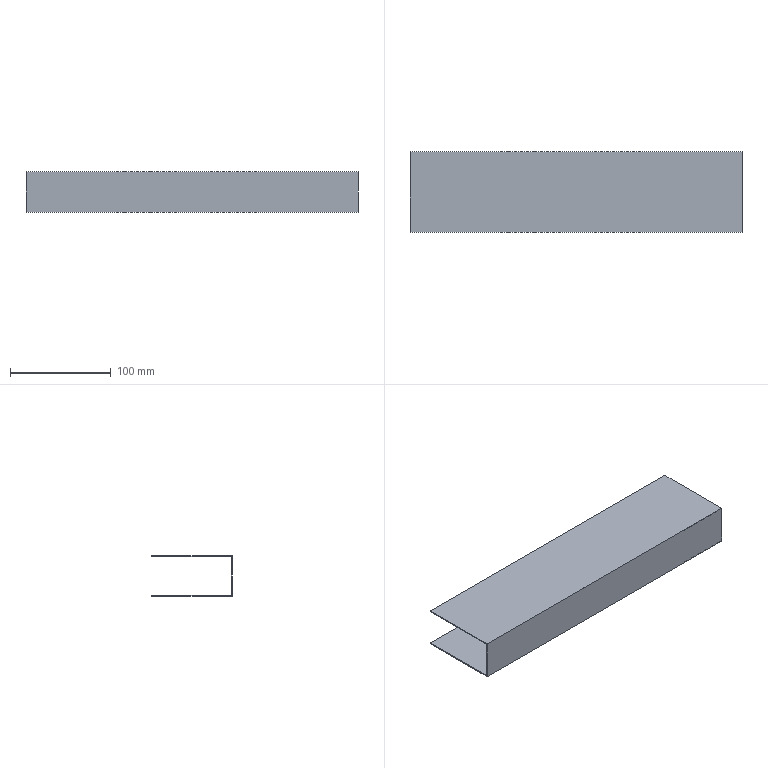Part | SolidWorks | features BaseBody 1 | 1 solid | 10 faces | box 330 x 80 x 40 mm | volume 65340 mm3 | plane 10
STEP:
#1=CARTESIAN_POINT('',(0.,1.,19.));
#2=VERTEX_POINT('',#1);
#3=CARTESIAN_POINT('',(0.,80.,19.));
#4=VERTEX_POINT('',#3);
#5=CARTESIAN_POINT('',(0.,0.,19.));
#6=DIRECTION('',(0.,1.,0.));
#7=VECTOR('',#6,1000.);
#8=LINE('',#5,#7);
#9=EDGE_CURVE('',#2,#4,#8,.T.);
#10=ORIENTED_EDGE('',*,*,#9,.F.);
#11=CARTESIAN_POINT('',(0.,1.,-19.));
#12=VERTEX_POINT('',#11);
#13=CARTESIAN_POINT('',(0.,1.,20.));
#14=DIRECTION('',(0.,0.,1.));
#15=VECTOR('',#14,1000.);
#16=LINE('',#13,#15);
#17=EDGE_CURVE('',#12,#2,#16,.T.);
#18=ORIENTED_EDGE('',*,*,#17,.F.);
#19=CARTESIAN_POINT('',(0.,80.,-19.));
#20=VERTEX_POINT('',#19);
#21=CARTESIAN_POINT('',(0.,0.,-19.));
#22=DIRECTION('',(0.,-1.,0.));
#23=VECTOR('',#22,1000.);
#24=LINE('',#21,#23);
#25=EDGE_CURVE('',#20,#12,#24,.T.);
#26=ORIENTED_EDGE('',*,*,#25,.F.);
#27=CARTESIAN_POINT('',(0.,80.,-20.));
#28=VERTEX_POINT('',#27);
#29=CARTESIAN_POINT('',(0.,80.,-19.));
#30=DIRECTION('',(0.,0.,-1.));
#31=VECTOR('',#30,1000.);
#32=LINE('',#29,#31);
#33=EDGE_CURVE('',#20,#28,#32,.T.);
#34=ORIENTED_EDGE('',*,*,#33,.T.);
#35=CARTESIAN_POINT('',(0.,0.,-20.));
#36=VERTEX_POINT('',#35);
#37=CARTESIAN_POINT('',(0.,0.,-20.));
#38=DIRECTION('',(0.,-1.,0.));
#39=VECTOR('',#38,1000.);
#40=LINE('',#37,#39);
#41=EDGE_CURVE('',#28,#36,#40,.T.);
#42=ORIENTED_EDGE('',*,*,#41,.T.);
#43=CARTESIAN_POINT('',(0.,0.,20.));
#44=VERTEX_POINT('',#43);
#45=CARTESIAN_POINT('',(0.,0.,20.));
#46=DIRECTION('',(0.,0.,1.));
#47=VECTOR('',#46,1000.);
#48=LINE('',#45,#47);
#49=EDGE_CURVE('',#36,#44,#48,.T.);
#50=ORIENTED_EDGE('',*,*,#49,.T.);
#51=CARTESIAN_POINT('',(0.,80.,20.));
#52=VERTEX_POINT('',#51);
#53=CARTESIAN_POINT('',(0.,0.,20.));
#54=DIRECTION('',(0.,1.,0.));
#55=VECTOR('',#54,1000.);
#56=LINE('',#53,#55);
#57=EDGE_CURVE('',#44,#52,#56,.T.);
#58=ORIENTED_EDGE('',*,*,#57,.T.);
#59=CARTESIAN_POINT('',(0.,80.,20.));
#60=DIRECTION('',(0.,0.,-1.));
#61=VECTOR('',#60,1000.);
#62=LINE('',#59,#61);
#63=EDGE_CURVE('',#52,#4,#62,.T.);
#64=ORIENTED_EDGE('',*,*,#63,.T.);
#65=EDGE_LOOP('',(#10,#18,#26,#34,#42,#50,#58,#64));
#66=FACE_OUTER_BOUND('',#65,.T.);
#67=CARTESIAN_POINT('',(0.,0.,0.));
#68=DIRECTION('',(-1.,0.,0.));
#69=DIRECTION('',(0.,0.,1.));
#70=AXIS2_PLACEMENT_3D('',#67,#68,#69);
#71=PLANE('',#70);
#72=ADVANCED_FACE('',(#66),#71,.T.);
#73=CARTESIAN_POINT('',(330.,1.,19.));
#74=VERTEX_POINT('',#73);
#75=CARTESIAN_POINT('',(330.,80.,19.));
#76=VERTEX_POINT('',#75);
#77=CARTESIAN_POINT('',(330.,0.,19.));
#78=DIRECTION('',(0.,1.,0.));
#79=VECTOR('',#78,1000.);
#80=LINE('',#77,#79);
#81=EDGE_CURVE('',#74,#76,#80,.T.);
#82=ORIENTED_EDGE('',*,*,#81,.T.);
#83=CARTESIAN_POINT('',(330.,80.,20.));
#84=VERTEX_POINT('',#83);
#85=CARTESIAN_POINT('',(330.,80.,20.));
#86=DIRECTION('',(0.,0.,-1.));
#87=VECTOR('',#86,1000.);
#88=LINE('',#85,#87);
#89=EDGE_CURVE('',#84,#76,#88,.T.);
#90=ORIENTED_EDGE('',*,*,#89,.F.);
#91=CARTESIAN_POINT('',(330.,0.,20.));
#92=VERTEX_POINT('',#91);
#93=CARTESIAN_POINT('',(330.,0.,20.));
#94=DIRECTION('',(0.,1.,0.));
#95=VECTOR('',#94,1000.);
#96=LINE('',#93,#95);
#97=EDGE_CURVE('',#92,#84,#96,.T.);
#98=ORIENTED_EDGE('',*,*,#97,.F.);
#99=CARTESIAN_POINT('',(330.,0.,-20.));
#100=VERTEX_POINT('',#99);
#101=CARTESIAN_POINT('',(330.,0.,20.));
#102=DIRECTION('',(0.,0.,1.));
#103=VECTOR('',#102,1000.);
#104=LINE('',#101,#103);
#105=EDGE_CURVE('',#100,#92,#104,.T.);
#106=ORIENTED_EDGE('',*,*,#105,.F.);
#107=CARTESIAN_POINT('',(330.,80.,-20.));
#108=VERTEX_POINT('',#107);
#109=CARTESIAN_POINT('',(330.,0.,-20.));
#110=DIRECTION('',(0.,-1.,0.));
#111=VECTOR('',#110,1000.);
#112=LINE('',#109,#111);
#113=EDGE_CURVE('',#108,#100,#112,.T.);
#114=ORIENTED_EDGE('',*,*,#113,.F.);
#115=CARTESIAN_POINT('',(330.,80.,-19.));
#116=VERTEX_POINT('',#115);
#117=CARTESIAN_POINT('',(330.,80.,-19.));
#118=DIRECTION('',(0.,0.,-1.));
#119=VECTOR('',#118,1000.);
#120=LINE('',#117,#119);
#121=EDGE_CURVE('',#116,#108,#120,.T.);
#122=ORIENTED_EDGE('',*,*,#121,.F.);
#123=CARTESIAN_POINT('',(330.,1.,-19.));
#124=VERTEX_POINT('',#123);
#125=CARTESIAN_POINT('',(330.,0.,-19.));
#126=DIRECTION('',(0.,-1.,0.));
#127=VECTOR('',#126,1000.);
#128=LINE('',#125,#127);
#129=EDGE_CURVE('',#116,#124,#128,.T.);
#130=ORIENTED_EDGE('',*,*,#129,.T.);
#131=CARTESIAN_POINT('',(330.,1.,20.));
#132=DIRECTION('',(0.,0.,1.));
#133=VECTOR('',#132,1000.);
#134=LINE('',#131,#133);
#135=EDGE_CURVE('',#124,#74,#134,.T.);
#136=ORIENTED_EDGE('',*,*,#135,.T.);
#137=EDGE_LOOP('',(#82,#90,#98,#106,#114,#122,#130,#136));
#138=FACE_OUTER_BOUND('',#137,.T.);
#139=CARTESIAN_POINT('',(330.,0.,0.));
#140=DIRECTION('',(-1.,0.,0.));
#141=DIRECTION('',(0.,0.,1.));
#142=AXIS2_PLACEMENT_3D('',#139,#140,#141);
#143=PLANE('',#142);
#144=ADVANCED_FACE('',(#138),#143,.F.);
#145=ORIENTED_EDGE('',*,*,#17,.T.);
#146=CARTESIAN_POINT('',(330.,1.,19.));
#147=DIRECTION('',(-1.,0.,0.));
#148=VECTOR('',#147,1000.);
#149=LINE('',#146,#148);
#150=EDGE_CURVE('',#74,#2,#149,.T.);
#151=ORIENTED_EDGE('',*,*,#150,.F.);
#152=ORIENTED_EDGE('',*,*,#135,.F.);
#153=CARTESIAN_POINT('',(330.,1.,-19.));
#154=DIRECTION('',(-1.,0.,0.));
#155=VECTOR('',#154,1000.);
#156=LINE('',#153,#155);
#157=EDGE_CURVE('',#124,#12,#156,.T.);
#158=ORIENTED_EDGE('',*,*,#157,.T.);
#159=EDGE_LOOP('',(#145,#151,#152,#158));
#160=FACE_OUTER_BOUND('',#159,.T.);
#161=CARTESIAN_POINT('',(330.,1.,20.));
#162=DIRECTION('',(0.,-1.,0.));
#163=DIRECTION('',(0.,0.,-1.));
#164=AXIS2_PLACEMENT_3D('',#161,#162,#163);
#165=PLANE('',#164);
#166=ADVANCED_FACE('',(#160),#165,.F.);
#167=ORIENTED_EDGE('',*,*,#25,.T.);
#168=ORIENTED_EDGE('',*,*,#157,.F.);
#169=ORIENTED_EDGE('',*,*,#129,.F.);
#170=CARTESIAN_POINT('',(330.,80.,-19.));
#171=DIRECTION('',(-1.,0.,0.));
#172=VECTOR('',#171,1000.);
#173=LINE('',#170,#172);
#174=EDGE_CURVE('',#116,#20,#173,.T.);
#175=ORIENTED_EDGE('',*,*,#174,.T.);
#176=EDGE_LOOP('',(#167,#168,#169,#175));
#177=FACE_OUTER_BOUND('',#176,.T.);
#178=CARTESIAN_POINT('',(330.,0.,-19.));
#179=DIRECTION('',(0.,0.,-1.));
#180=DIRECTION('',(0.,-1.,0.));
#181=AXIS2_PLACEMENT_3D('',#178,#179,#180);
#182=PLANE('',#181);
#183=ADVANCED_FACE('',(#177),#182,.F.);
#184=ORIENTED_EDGE('',*,*,#33,.F.);
#185=ORIENTED_EDGE('',*,*,#174,.F.);
#186=ORIENTED_EDGE('',*,*,#121,.T.);
#187=CARTESIAN_POINT('',(330.,80.,-20.));
#188=DIRECTION('',(-1.,0.,0.));
#189=VECTOR('',#188,1000.);
#190=LINE('',#187,#189);
#191=EDGE_CURVE('',#108,#28,#190,.T.);
#192=ORIENTED_EDGE('',*,*,#191,.T.);
#193=EDGE_LOOP('',(#184,#185,#186,#192));
#194=FACE_OUTER_BOUND('',#193,.T.);
#195=CARTESIAN_POINT('',(330.,80.,-19.));
#196=DIRECTION('',(0.,1.,0.));
#197=DIRECTION('',(1.,0.,0.));
#198=AXIS2_PLACEMENT_3D('',#195,#196,#197);
#199=PLANE('',#198);
#200=ADVANCED_FACE('',(#194),#199,.T.);
#201=ORIENTED_EDGE('',*,*,#41,.F.);
#202=ORIENTED_EDGE('',*,*,#191,.F.);
#203=ORIENTED_EDGE('',*,*,#113,.T.);
#204=CARTESIAN_POINT('',(330.,0.,-20.));
#205=DIRECTION('',(-1.,0.,0.));
#206=VECTOR('',#205,1000.);
#207=LINE('',#204,#206);
#208=EDGE_CURVE('',#100,#36,#207,.T.);
#209=ORIENTED_EDGE('',*,*,#208,.T.);
#210=EDGE_LOOP('',(#201,#202,#203,#209));
#211=FACE_OUTER_BOUND('',#210,.T.);
#212=CARTESIAN_POINT('',(330.,0.,-20.));
#213=DIRECTION('',(0.,0.,-1.));
#214=DIRECTION('',(0.,-1.,0.));
#215=AXIS2_PLACEMENT_3D('',#212,#213,#214);
#216=PLANE('',#215);
#217=ADVANCED_FACE('',(#211),#216,.T.);
#218=ORIENTED_EDGE('',*,*,#49,.F.);
#219=ORIENTED_EDGE('',*,*,#208,.F.);
#220=ORIENTED_EDGE('',*,*,#105,.T.);
#221=CARTESIAN_POINT('',(330.,0.,20.));
#222=DIRECTION('',(-1.,0.,0.));
#223=VECTOR('',#222,1000.);
#224=LINE('',#221,#223);
#225=EDGE_CURVE('',#92,#44,#224,.T.);
#226=ORIENTED_EDGE('',*,*,#225,.T.);
#227=EDGE_LOOP('',(#218,#219,#220,#226));
#228=FACE_OUTER_BOUND('',#227,.T.);
#229=CARTESIAN_POINT('',(330.,0.,20.));
#230=DIRECTION('',(0.,-1.,0.));
#231=DIRECTION('',(0.,0.,-1.));
#232=AXIS2_PLACEMENT_3D('',#229,#230,#231);
#233=PLANE('',#232);
#234=ADVANCED_FACE('',(#228),#233,.T.);
#235=ORIENTED_EDGE('',*,*,#57,.F.);
#236=ORIENTED_EDGE('',*,*,#225,.F.);
#237=ORIENTED_EDGE('',*,*,#97,.T.);
#238=CARTESIAN_POINT('',(330.,80.,20.));
#239=DIRECTION('',(-1.,0.,0.));
#240=VECTOR('',#239,1000.);
#241=LINE('',#238,#240);
#242=EDGE_CURVE('',#84,#52,#241,.T.);
#243=ORIENTED_EDGE('',*,*,#242,.T.);
#244=EDGE_LOOP('',(#235,#236,#237,#243));
#245=FACE_OUTER_BOUND('',#244,.T.);
#246=CARTESIAN_POINT('',(330.,0.,20.));
#247=DIRECTION('',(0.,0.,1.));
#248=DIRECTION('',(0.,-1.,0.));
#249=AXIS2_PLACEMENT_3D('',#246,#247,#248);
#250=PLANE('',#249);
#251=ADVANCED_FACE('',(#245),#250,.T.);
#252=ORIENTED_EDGE('',*,*,#63,.F.);
#253=ORIENTED_EDGE('',*,*,#242,.F.);
#254=ORIENTED_EDGE('',*,*,#89,.T.);
#255=CARTESIAN_POINT('',(330.,80.,19.));
#256=DIRECTION('',(-1.,0.,0.));
#257=VECTOR('',#256,1000.);
#258=LINE('',#255,#257);
#259=EDGE_CURVE('',#76,#4,#258,.T.);
#260=ORIENTED_EDGE('',*,*,#259,.T.);
#261=EDGE_LOOP('',(#252,#253,#254,#260));
#262=FACE_OUTER_BOUND('',#261,.T.);
#263=CARTESIAN_POINT('',(330.,80.,20.));
#264=DIRECTION('',(0.,1.,0.));
#265=DIRECTION('',(1.,0.,0.));
#266=AXIS2_PLACEMENT_3D('',#263,#264,#265);
#267=PLANE('',#266);
#268=ADVANCED_FACE('',(#262),#267,.T.);
#269=ORIENTED_EDGE('',*,*,#9,.T.);
#270=ORIENTED_EDGE('',*,*,#259,.F.);
#271=ORIENTED_EDGE('',*,*,#81,.F.);
#272=ORIENTED_EDGE('',*,*,#150,.T.);
#273=EDGE_LOOP('',(#269,#270,#271,#272));
#274=FACE_OUTER_BOUND('',#273,.T.);
#275=CARTESIAN_POINT('',(330.,0.,19.));
#276=DIRECTION('',(0.,0.,1.));
#277=DIRECTION('',(0.,-1.,0.));
#278=AXIS2_PLACEMENT_3D('',#275,#276,#277);
#279=PLANE('',#278);
#280=ADVANCED_FACE('',(#274),#279,.F.);
#281=CLOSED_SHELL('',(#72,#144,#166,#183,#200,#217,#234,#251,#268,#280));
#282=MANIFOLD_SOLID_BREP('',#281);
#283=CARTESIAN_POINT('',(0.,0.,0.));
#284=DIRECTION('',(0.,0.,1.));
#285=DIRECTION('',(1.,0.,0.));
#286=AXIS2_PLACEMENT_3D('',#283,#284,#285);
#287=(LENGTH_UNIT()NAMED_UNIT(*)SI_UNIT(.MILLI.,.METRE.));
#288=UNCERTAINTY_MEASURE_WITH_UNIT(LENGTH_MEASURE(0.00001),#287,'','');
#289=(NAMED_UNIT(*)PLANE_ANGLE_UNIT()SI_UNIT($,.RADIAN.));
#290=(NAMED_UNIT(*)SI_UNIT($,.STERADIAN.)SOLID_ANGLE_UNIT());
#291=(GEOMETRIC_REPRESENTATION_CONTEXT(3)GLOBAL_UNCERTAINTY_ASSIGNED_CONTEXT((#288))GLOBAL_UNIT_ASSIGNED_CONTEXT((#287,#289,#290))REPRESENTATION_CONTEXT('',''));
#292=ADVANCED_BREP_SHAPE_REPRESENTATION('',(#282,#286),#291);